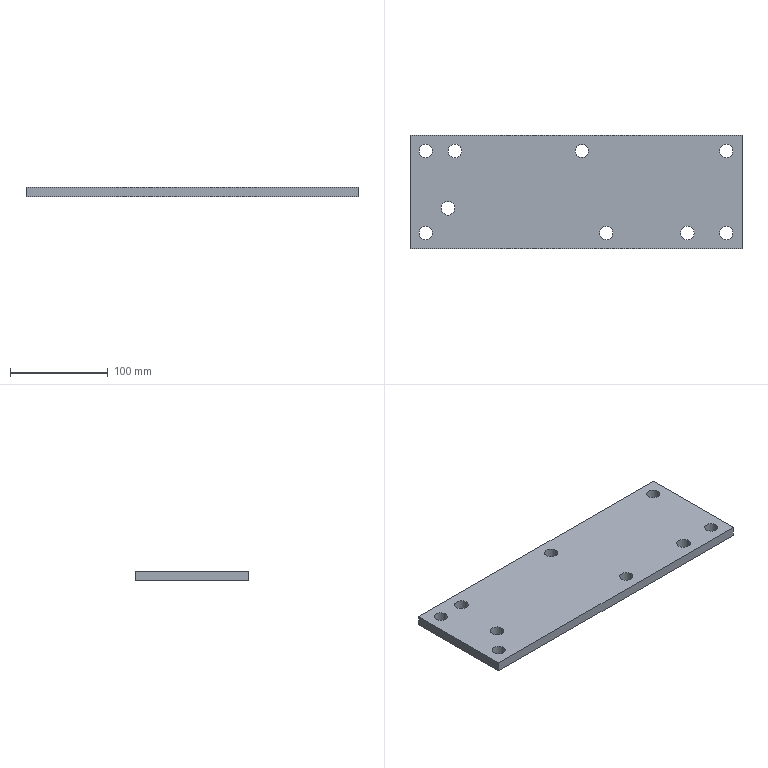Part | NX | features 6 2 | 1 solid | 15 faces | box 340 x 116 x 10 mm | volume 381193 mm3 | cylinder 9 | plane 6 | commonest cylinder face diameters 13.5 x6 14.001 x2 14 x1
STEP:
#1=CARTESIAN_POINT('',(268.029,-411.95,91.));
#2=VERTEX_POINT('',#1);
#3=CARTESIAN_POINT('',(275.029,-411.95,91.));
#4=DIRECTION('',(0.,0.,1.));
#5=DIRECTION('',(-1.,0.,0.));
#6=AXIS2_PLACEMENT_3D('',#3,#4,#5);
#7=CIRCLE('',#6,7.);
#8=EDGE_CURVE('',#2,#2,#7,.T.);
#9=ORIENTED_EDGE('',*,*,#8,.T.);
#10=EDGE_LOOP('',(#9));
#11=FACE_BOUND('',#10,.T.);
#12=CARTESIAN_POINT('',(405.359,-353.223,91.));
#13=VERTEX_POINT('',#12);
#14=CARTESIAN_POINT('',(412.109,-353.223,91.));
#15=DIRECTION('',(0.,0.,-1.));
#16=DIRECTION('',(-1.,0.,0.));
#17=AXIS2_PLACEMENT_3D('',#14,#15,#16);
#18=CIRCLE('',#17,6.75);
#19=EDGE_CURVE('',#13,#13,#18,.T.);
#20=ORIENTED_EDGE('',*,*,#19,.F.);
#21=EDGE_LOOP('',(#20));
#22=FACE_BOUND('',#21,.T.);
#23=CARTESIAN_POINT('',(430.359,-437.223,91.));
#24=VERTEX_POINT('',#23);
#25=CARTESIAN_POINT('',(437.109,-437.223,91.));
#26=DIRECTION('',(0.,0.,-1.));
#27=DIRECTION('',(-1.,0.,0.));
#28=AXIS2_PLACEMENT_3D('',#25,#26,#27);
#29=CIRCLE('',#28,6.75);
#30=EDGE_CURVE('',#24,#24,#29,.T.);
#31=ORIENTED_EDGE('',*,*,#30,.F.);
#32=EDGE_LOOP('',(#31));
#33=FACE_BOUND('',#32,.T.);
#34=CARTESIAN_POINT('',(289.11,-353.223,91.));
#35=VERTEX_POINT('',#34);
#36=CARTESIAN_POINT('',(282.109,-353.223,91.));
#37=DIRECTION('',(0.,0.,-1.));
#38=DIRECTION('',(1.,0.,0.));
#39=AXIS2_PLACEMENT_3D('',#36,#37,#38);
#40=CIRCLE('',#39,7.);
#41=EDGE_CURVE('',#35,#35,#40,.T.);
#42=ORIENTED_EDGE('',*,*,#41,.F.);
#43=EDGE_LOOP('',(#42));
#44=FACE_BOUND('',#43,.T.);
#45=CARTESIAN_POINT('',(566.859,-353.223,91.));
#46=VERTEX_POINT('',#45);
#47=CARTESIAN_POINT('',(560.109,-353.223,91.));
#48=DIRECTION('',(0.,0.,-1.));
#49=DIRECTION('',(1.,0.,0.));
#50=AXIS2_PLACEMENT_3D('',#47,#48,#49);
#51=CIRCLE('',#50,6.75);
#52=EDGE_CURVE('',#46,#46,#51,.T.);
#53=ORIENTED_EDGE('',*,*,#52,.F.);
#54=EDGE_LOOP('',(#53));
#55=FACE_BOUND('',#54,.T.);
#56=CARTESIAN_POINT('',(258.859,-353.223,91.));
#57=VERTEX_POINT('',#56);
#58=CARTESIAN_POINT('',(252.109,-353.223,91.));
#59=DIRECTION('',(0.,0.,-1.));
#60=DIRECTION('',(1.,0.,0.));
#61=AXIS2_PLACEMENT_3D('',#58,#59,#60);
#62=CIRCLE('',#61,6.75);
#63=EDGE_CURVE('',#57,#57,#62,.T.);
#64=ORIENTED_EDGE('',*,*,#63,.F.);
#65=EDGE_LOOP('',(#64));
#66=FACE_BOUND('',#65,.T.);
#67=CARTESIAN_POINT('',(576.109,-337.223,91.));
#68=VERTEX_POINT('',#67);
#69=CARTESIAN_POINT('',(576.109,-453.223,91.));
#70=VERTEX_POINT('',#69);
#71=CARTESIAN_POINT('',(576.109,-392.723,91.));
#72=DIRECTION('',(0.,-1.,0.));
#73=VECTOR('',#72,1000.);
#74=LINE('',#71,#73);
#75=EDGE_CURVE('',#68,#70,#74,.T.);
#76=ORIENTED_EDGE('',*,*,#75,.T.);
#77=CARTESIAN_POINT('',(236.109,-453.223,91.));
#78=VERTEX_POINT('',#77);
#79=CARTESIAN_POINT('',(433.109,-453.223,91.));
#80=DIRECTION('',(-1.,0.,0.));
#81=VECTOR('',#80,1000.);
#82=LINE('',#79,#81);
#83=EDGE_CURVE('',#70,#78,#82,.T.);
#84=ORIENTED_EDGE('',*,*,#83,.T.);
#85=CARTESIAN_POINT('',(236.109,-337.223,91.));
#86=VERTEX_POINT('',#85);
#87=CARTESIAN_POINT('',(236.109,-392.723,91.));
#88=DIRECTION('',(0.,1.,0.));
#89=VECTOR('',#88,1000.);
#90=LINE('',#87,#89);
#91=EDGE_CURVE('',#78,#86,#90,.T.);
#92=ORIENTED_EDGE('',*,*,#91,.T.);
#93=CARTESIAN_POINT('',(433.109,-337.223,91.));
#94=DIRECTION('',(1.,0.,0.));
#95=VECTOR('',#94,1000.);
#96=LINE('',#93,#95);
#97=EDGE_CURVE('',#86,#68,#96,.T.);
#98=ORIENTED_EDGE('',*,*,#97,.T.);
#99=EDGE_LOOP('',(#76,#84,#92,#98));
#100=FACE_BOUND('',#99,.T.);
#101=CARTESIAN_POINT('',(566.859,-437.223,91.));
#102=VERTEX_POINT('',#101);
#103=CARTESIAN_POINT('',(560.109,-437.223,91.));
#104=DIRECTION('',(0.,0.,-1.));
#105=DIRECTION('',(1.,0.,0.));
#106=AXIS2_PLACEMENT_3D('',#103,#104,#105);
#107=CIRCLE('',#106,6.75);
#108=EDGE_CURVE('',#102,#102,#107,.T.);
#109=ORIENTED_EDGE('',*,*,#108,.F.);
#110=EDGE_LOOP('',(#109));
#111=FACE_BOUND('',#110,.T.);
#112=CARTESIAN_POINT('',(258.859,-437.223,91.));
#113=VERTEX_POINT('',#112);
#114=CARTESIAN_POINT('',(252.109,-437.223,91.));
#115=DIRECTION('',(0.,0.,-1.));
#116=DIRECTION('',(1.,0.,0.));
#117=AXIS2_PLACEMENT_3D('',#114,#115,#116);
#118=CIRCLE('',#117,6.75);
#119=EDGE_CURVE('',#113,#113,#118,.T.);
#120=ORIENTED_EDGE('',*,*,#119,.F.);
#121=EDGE_LOOP('',(#120));
#122=FACE_BOUND('',#121,.T.);
#123=CARTESIAN_POINT('',(527.11,-437.223,91.));
#124=VERTEX_POINT('',#123);
#125=CARTESIAN_POINT('',(520.109,-437.223,91.));
#126=DIRECTION('',(0.,0.,-1.));
#127=DIRECTION('',(1.,0.,0.));
#128=AXIS2_PLACEMENT_3D('',#125,#126,#127);
#129=CIRCLE('',#128,7.);
#130=EDGE_CURVE('',#124,#124,#129,.T.);
#131=ORIENTED_EDGE('',*,*,#130,.F.);
#132=EDGE_LOOP('',(#131));
#133=FACE_BOUND('',#132,.T.);
#134=CARTESIAN_POINT('',(433.109,-392.723,91.));
#135=DIRECTION('',(0.,0.,-1.));
#136=DIRECTION('',(1.,0.,0.));
#137=AXIS2_PLACEMENT_3D('',#134,#135,#136);
#138=PLANE('',#137);
#139=ADVANCED_FACE('',(#11,#22,#33,#44,#55,#66,#100,#111,#122,#133),#138,.T.);
#140=CARTESIAN_POINT('',(282.029,-411.95,101.));
#141=VERTEX_POINT('',#140);
#142=CARTESIAN_POINT('',(275.029,-411.95,101.));
#143=DIRECTION('',(0.,0.,-1.));
#144=DIRECTION('',(1.,0.,0.));
#145=AXIS2_PLACEMENT_3D('',#142,#143,#144);
#146=CIRCLE('',#145,7.);
#147=EDGE_CURVE('',#141,#141,#146,.T.);
#148=ORIENTED_EDGE('',*,*,#147,.T.);
#149=EDGE_LOOP('',(#148));
#150=FACE_BOUND('',#149,.T.);
#151=CARTESIAN_POINT('',(418.859,-353.223,101.));
#152=VERTEX_POINT('',#151);
#153=CARTESIAN_POINT('',(412.109,-353.223,101.));
#154=DIRECTION('',(0.,0.,1.));
#155=DIRECTION('',(1.,0.,0.));
#156=AXIS2_PLACEMENT_3D('',#153,#154,#155);
#157=CIRCLE('',#156,6.75);
#158=EDGE_CURVE('',#152,#152,#157,.T.);
#159=ORIENTED_EDGE('',*,*,#158,.F.);
#160=EDGE_LOOP('',(#159));
#161=FACE_BOUND('',#160,.T.);
#162=CARTESIAN_POINT('',(443.859,-437.223,101.));
#163=VERTEX_POINT('',#162);
#164=CARTESIAN_POINT('',(437.109,-437.223,101.));
#165=DIRECTION('',(0.,0.,1.));
#166=DIRECTION('',(1.,0.,0.));
#167=AXIS2_PLACEMENT_3D('',#164,#165,#166);
#168=CIRCLE('',#167,6.75);
#169=EDGE_CURVE('',#163,#163,#168,.T.);
#170=ORIENTED_EDGE('',*,*,#169,.F.);
#171=EDGE_LOOP('',(#170));
#172=FACE_BOUND('',#171,.T.);
#173=CARTESIAN_POINT('',(289.11,-353.223,101.));
#174=VERTEX_POINT('',#173);
#175=CARTESIAN_POINT('',(282.109,-353.223,101.));
#176=DIRECTION('',(0.,0.,1.));
#177=DIRECTION('',(1.,0.,0.));
#178=AXIS2_PLACEMENT_3D('',#175,#176,#177);
#179=CIRCLE('',#178,7.);
#180=EDGE_CURVE('',#174,#174,#179,.T.);
#181=ORIENTED_EDGE('',*,*,#180,.F.);
#182=EDGE_LOOP('',(#181));
#183=FACE_BOUND('',#182,.T.);
#184=CARTESIAN_POINT('',(566.859,-353.223,101.));
#185=VERTEX_POINT('',#184);
#186=CARTESIAN_POINT('',(560.109,-353.223,101.));
#187=DIRECTION('',(0.,0.,1.));
#188=DIRECTION('',(1.,0.,0.));
#189=AXIS2_PLACEMENT_3D('',#186,#187,#188);
#190=CIRCLE('',#189,6.75);
#191=EDGE_CURVE('',#185,#185,#190,.T.);
#192=ORIENTED_EDGE('',*,*,#191,.F.);
#193=EDGE_LOOP('',(#192));
#194=FACE_BOUND('',#193,.T.);
#195=CARTESIAN_POINT('',(258.859,-353.223,101.));
#196=VERTEX_POINT('',#195);
#197=CARTESIAN_POINT('',(252.109,-353.223,101.));
#198=DIRECTION('',(0.,0.,1.));
#199=DIRECTION('',(1.,0.,0.));
#200=AXIS2_PLACEMENT_3D('',#197,#198,#199);
#201=CIRCLE('',#200,6.75);
#202=EDGE_CURVE('',#196,#196,#201,.T.);
#203=ORIENTED_EDGE('',*,*,#202,.F.);
#204=EDGE_LOOP('',(#203));
#205=FACE_BOUND('',#204,.T.);
#206=CARTESIAN_POINT('',(576.109,-337.223,101.));
#207=VERTEX_POINT('',#206);
#208=CARTESIAN_POINT('',(236.109,-337.223,101.));
#209=VERTEX_POINT('',#208);
#210=CARTESIAN_POINT('',(433.109,-337.223,101.));
#211=DIRECTION('',(-1.,0.,0.));
#212=VECTOR('',#211,1000.);
#213=LINE('',#210,#212);
#214=EDGE_CURVE('',#207,#209,#213,.T.);
#215=ORIENTED_EDGE('',*,*,#214,.T.);
#216=CARTESIAN_POINT('',(236.109,-453.223,101.));
#217=VERTEX_POINT('',#216);
#218=CARTESIAN_POINT('',(236.109,-392.723,101.));
#219=DIRECTION('',(0.,-1.,0.));
#220=VECTOR('',#219,1000.);
#221=LINE('',#218,#220);
#222=EDGE_CURVE('',#209,#217,#221,.T.);
#223=ORIENTED_EDGE('',*,*,#222,.T.);
#224=CARTESIAN_POINT('',(576.109,-453.223,101.));
#225=VERTEX_POINT('',#224);
#226=CARTESIAN_POINT('',(433.109,-453.223,101.));
#227=DIRECTION('',(1.,0.,0.));
#228=VECTOR('',#227,1000.);
#229=LINE('',#226,#228);
#230=EDGE_CURVE('',#217,#225,#229,.T.);
#231=ORIENTED_EDGE('',*,*,#230,.T.);
#232=CARTESIAN_POINT('',(576.109,-392.723,101.));
#233=DIRECTION('',(0.,1.,0.));
#234=VECTOR('',#233,1000.);
#235=LINE('',#232,#234);
#236=EDGE_CURVE('',#225,#207,#235,.T.);
#237=ORIENTED_EDGE('',*,*,#236,.T.);
#238=EDGE_LOOP('',(#215,#223,#231,#237));
#239=FACE_BOUND('',#238,.T.);
#240=CARTESIAN_POINT('',(566.859,-437.223,101.));
#241=VERTEX_POINT('',#240);
#242=CARTESIAN_POINT('',(560.109,-437.223,101.));
#243=DIRECTION('',(0.,0.,1.));
#244=DIRECTION('',(1.,0.,0.));
#245=AXIS2_PLACEMENT_3D('',#242,#243,#244);
#246=CIRCLE('',#245,6.75);
#247=EDGE_CURVE('',#241,#241,#246,.T.);
#248=ORIENTED_EDGE('',*,*,#247,.F.);
#249=EDGE_LOOP('',(#248));
#250=FACE_BOUND('',#249,.T.);
#251=CARTESIAN_POINT('',(258.859,-437.223,101.));
#252=VERTEX_POINT('',#251);
#253=CARTESIAN_POINT('',(252.109,-437.223,101.));
#254=DIRECTION('',(0.,0.,1.));
#255=DIRECTION('',(1.,0.,0.));
#256=AXIS2_PLACEMENT_3D('',#253,#254,#255);
#257=CIRCLE('',#256,6.75);
#258=EDGE_CURVE('',#252,#252,#257,.T.);
#259=ORIENTED_EDGE('',*,*,#258,.F.);
#260=EDGE_LOOP('',(#259));
#261=FACE_BOUND('',#260,.T.);
#262=CARTESIAN_POINT('',(527.11,-437.223,101.));
#263=VERTEX_POINT('',#262);
#264=CARTESIAN_POINT('',(520.109,-437.223,101.));
#265=DIRECTION('',(0.,0.,1.));
#266=DIRECTION('',(1.,0.,0.));
#267=AXIS2_PLACEMENT_3D('',#264,#265,#266);
#268=CIRCLE('',#267,7.);
#269=EDGE_CURVE('',#263,#263,#268,.T.);
#270=ORIENTED_EDGE('',*,*,#269,.F.);
#271=EDGE_LOOP('',(#270));
#272=FACE_BOUND('',#271,.T.);
#273=CARTESIAN_POINT('',(-273.37,-123.939,101.));
#274=DIRECTION('',(0.,0.,1.));
#275=DIRECTION('',(-1.,0.,0.));
#276=AXIS2_PLACEMENT_3D('',#273,#274,#275);
#277=PLANE('',#276);
#278=ADVANCED_FACE('',(#150,#161,#172,#183,#194,#205,#239,#250,#261,#272),#277,.T.);
#279=ORIENTED_EDGE('',*,*,#269,.T.);
#280=EDGE_LOOP('',(#279));
#281=FACE_BOUND('',#280,.T.);
#282=ORIENTED_EDGE('',*,*,#130,.T.);
#283=EDGE_LOOP('',(#282));
#284=FACE_BOUND('',#283,.T.);
#285=CARTESIAN_POINT('',(520.109,-437.223,91.));
#286=DIRECTION('',(0.,0.,1.));
#287=DIRECTION('',(-1.,0.,0.));
#288=AXIS2_PLACEMENT_3D('',#285,#286,#287);
#289=CYLINDRICAL_SURFACE('',#288,7.);
#290=ADVANCED_FACE('',(#281,#284),#289,.F.);
#291=ORIENTED_EDGE('',*,*,#258,.T.);
#292=EDGE_LOOP('',(#291));
#293=FACE_BOUND('',#292,.T.);
#294=ORIENTED_EDGE('',*,*,#119,.T.);
#295=EDGE_LOOP('',(#294));
#296=FACE_BOUND('',#295,.T.);
#297=CARTESIAN_POINT('',(252.109,-437.223,91.));
#298=DIRECTION('',(0.,0.,1.));
#299=DIRECTION('',(-1.,0.,0.));
#300=AXIS2_PLACEMENT_3D('',#297,#298,#299);
#301=CYLINDRICAL_SURFACE('',#300,6.75);
#302=ADVANCED_FACE('',(#293,#296),#301,.F.);
#303=ORIENTED_EDGE('',*,*,#247,.T.);
#304=EDGE_LOOP('',(#303));
#305=FACE_BOUND('',#304,.T.);
#306=ORIENTED_EDGE('',*,*,#108,.T.);
#307=EDGE_LOOP('',(#306));
#308=FACE_BOUND('',#307,.T.);
#309=CARTESIAN_POINT('',(560.109,-437.223,91.));
#310=DIRECTION('',(0.,0.,1.));
#311=DIRECTION('',(-1.,0.,0.));
#312=AXIS2_PLACEMENT_3D('',#309,#310,#311);
#313=CYLINDRICAL_SURFACE('',#312,6.75);
#314=ADVANCED_FACE('',(#305,#308),#313,.F.);
#315=CARTESIAN_POINT('',(576.109,-337.223,91.));
#316=DIRECTION('',(0.,0.,1.));
#317=VECTOR('',#316,1000.);
#318=LINE('',#315,#317);
#319=EDGE_CURVE('',#68,#207,#318,.T.);
#320=ORIENTED_EDGE('',*,*,#319,.F.);
#321=ORIENTED_EDGE('',*,*,#97,.F.);
#322=CARTESIAN_POINT('',(236.109,-337.223,91.));
#323=DIRECTION('',(0.,0.,1.));
#324=VECTOR('',#323,1000.);
#325=LINE('',#322,#324);
#326=EDGE_CURVE('',#86,#209,#325,.T.);
#327=ORIENTED_EDGE('',*,*,#326,.T.);
#328=ORIENTED_EDGE('',*,*,#214,.F.);
#329=EDGE_LOOP('',(#320,#321,#327,#328));
#330=FACE_BOUND('',#329,.T.);
#331=CARTESIAN_POINT('',(433.109,-337.223,91.));
#332=DIRECTION('',(0.,1.,0.));
#333=DIRECTION('',(0.,0.,1.));
#334=AXIS2_PLACEMENT_3D('',#331,#332,#333);
#335=PLANE('',#334);
#336=ADVANCED_FACE('',(#330),#335,.T.);
#337=ORIENTED_EDGE('',*,*,#326,.F.);
#338=ORIENTED_EDGE('',*,*,#91,.F.);
#339=CARTESIAN_POINT('',(236.109,-453.223,91.));
#340=DIRECTION('',(0.,0.,1.));
#341=VECTOR('',#340,1000.);
#342=LINE('',#339,#341);
#343=EDGE_CURVE('',#78,#217,#342,.T.);
#344=ORIENTED_EDGE('',*,*,#343,.T.);
#345=ORIENTED_EDGE('',*,*,#222,.F.);
#346=EDGE_LOOP('',(#337,#338,#344,#345));
#347=FACE_BOUND('',#346,.T.);
#348=CARTESIAN_POINT('',(236.109,-392.723,91.));
#349=DIRECTION('',(-1.,0.,0.));
#350=DIRECTION('',(0.,0.,-1.));
#351=AXIS2_PLACEMENT_3D('',#348,#349,#350);
#352=PLANE('',#351);
#353=ADVANCED_FACE('',(#347),#352,.T.);
#354=ORIENTED_EDGE('',*,*,#343,.F.);
#355=ORIENTED_EDGE('',*,*,#83,.F.);
#356=CARTESIAN_POINT('',(576.109,-453.223,91.));
#357=DIRECTION('',(0.,0.,1.));
#358=VECTOR('',#357,1000.);
#359=LINE('',#356,#358);
#360=EDGE_CURVE('',#70,#225,#359,.T.);
#361=ORIENTED_EDGE('',*,*,#360,.T.);
#362=ORIENTED_EDGE('',*,*,#230,.F.);
#363=EDGE_LOOP('',(#354,#355,#361,#362));
#364=FACE_BOUND('',#363,.T.);
#365=CARTESIAN_POINT('',(433.109,-453.223,91.));
#366=DIRECTION('',(0.,-1.,0.));
#367=DIRECTION('',(0.,0.,-1.));
#368=AXIS2_PLACEMENT_3D('',#365,#366,#367);
#369=PLANE('',#368);
#370=ADVANCED_FACE('',(#364),#369,.T.);
#371=ORIENTED_EDGE('',*,*,#75,.F.);
#372=ORIENTED_EDGE('',*,*,#319,.T.);
#373=ORIENTED_EDGE('',*,*,#236,.F.);
#374=ORIENTED_EDGE('',*,*,#360,.F.);
#375=EDGE_LOOP('',(#371,#372,#373,#374));
#376=FACE_BOUND('',#375,.T.);
#377=CARTESIAN_POINT('',(576.109,-392.723,91.));
#378=DIRECTION('',(1.,0.,0.));
#379=DIRECTION('',(0.,0.,1.));
#380=AXIS2_PLACEMENT_3D('',#377,#378,#379);
#381=PLANE('',#380);
#382=ADVANCED_FACE('',(#376),#381,.T.);
#383=ORIENTED_EDGE('',*,*,#202,.T.);
#384=EDGE_LOOP('',(#383));
#385=FACE_BOUND('',#384,.T.);
#386=ORIENTED_EDGE('',*,*,#63,.T.);
#387=EDGE_LOOP('',(#386));
#388=FACE_BOUND('',#387,.T.);
#389=CARTESIAN_POINT('',(252.109,-353.223,91.));
#390=DIRECTION('',(0.,0.,1.));
#391=DIRECTION('',(-1.,0.,0.));
#392=AXIS2_PLACEMENT_3D('',#389,#390,#391);
#393=CYLINDRICAL_SURFACE('',#392,6.75);
#394=ADVANCED_FACE('',(#385,#388),#393,.F.);
#395=ORIENTED_EDGE('',*,*,#191,.T.);
#396=EDGE_LOOP('',(#395));
#397=FACE_BOUND('',#396,.T.);
#398=ORIENTED_EDGE('',*,*,#52,.T.);
#399=EDGE_LOOP('',(#398));
#400=FACE_BOUND('',#399,.T.);
#401=CARTESIAN_POINT('',(560.109,-353.223,91.));
#402=DIRECTION('',(0.,0.,1.));
#403=DIRECTION('',(-1.,0.,0.));
#404=AXIS2_PLACEMENT_3D('',#401,#402,#403);
#405=CYLINDRICAL_SURFACE('',#404,6.75);
#406=ADVANCED_FACE('',(#397,#400),#405,.F.);
#407=ORIENTED_EDGE('',*,*,#180,.T.);
#408=EDGE_LOOP('',(#407));
#409=FACE_BOUND('',#408,.T.);
#410=ORIENTED_EDGE('',*,*,#41,.T.);
#411=EDGE_LOOP('',(#410));
#412=FACE_BOUND('',#411,.T.);
#413=CARTESIAN_POINT('',(282.109,-353.223,91.));
#414=DIRECTION('',(0.,0.,1.));
#415=DIRECTION('',(-1.,0.,0.));
#416=AXIS2_PLACEMENT_3D('',#413,#414,#415);
#417=CYLINDRICAL_SURFACE('',#416,7.);
#418=ADVANCED_FACE('',(#409,#412),#417,.F.);
#419=ORIENTED_EDGE('',*,*,#169,.T.);
#420=EDGE_LOOP('',(#419));
#421=FACE_BOUND('',#420,.T.);
#422=ORIENTED_EDGE('',*,*,#30,.T.);
#423=EDGE_LOOP('',(#422));
#424=FACE_BOUND('',#423,.T.);
#425=CARTESIAN_POINT('',(437.109,-437.223,91.));
#426=DIRECTION('',(0.,0.,1.));
#427=DIRECTION('',(-1.,0.,0.));
#428=AXIS2_PLACEMENT_3D('',#425,#426,#427);
#429=CYLINDRICAL_SURFACE('',#428,6.75);
#430=ADVANCED_FACE('',(#421,#424),#429,.F.);
#431=ORIENTED_EDGE('',*,*,#158,.T.);
#432=EDGE_LOOP('',(#431));
#433=FACE_BOUND('',#432,.T.);
#434=ORIENTED_EDGE('',*,*,#19,.T.);
#435=EDGE_LOOP('',(#434));
#436=FACE_BOUND('',#435,.T.);
#437=CARTESIAN_POINT('',(412.109,-353.223,91.));
#438=DIRECTION('',(0.,0.,1.));
#439=DIRECTION('',(-1.,0.,0.));
#440=AXIS2_PLACEMENT_3D('',#437,#438,#439);
#441=CYLINDRICAL_SURFACE('',#440,6.75);
#442=ADVANCED_FACE('',(#433,#436),#441,.F.);
#443=ORIENTED_EDGE('',*,*,#8,.F.);
#444=EDGE_LOOP('',(#443));
#445=FACE_BOUND('',#444,.T.);
#446=ORIENTED_EDGE('',*,*,#147,.F.);
#447=EDGE_LOOP('',(#446));
#448=FACE_BOUND('',#447,.T.);
#449=CARTESIAN_POINT('',(275.029,-411.95,-138.15));
#450=DIRECTION('',(0.,0.,1.));
#451=DIRECTION('',(-1.,0.,0.));
#452=AXIS2_PLACEMENT_3D('',#449,#450,#451);
#453=CYLINDRICAL_SURFACE('',#452,7.);
#454=ADVANCED_FACE('',(#445,#448),#453,.F.);
#455=CLOSED_SHELL('',(#139,#278,#290,#302,#314,#336,#353,#370,#382,#394,#406,#418,#430,#442,#454));
#456=MANIFOLD_SOLID_BREP('',#455);
#457=(LENGTH_UNIT()NAMED_UNIT(*)SI_UNIT(.MILLI.,.METRE.));
#458=UNCERTAINTY_MEASURE_WITH_UNIT(LENGTH_MEASURE(0.00001),#457,'','');
#459=(NAMED_UNIT(*)PLANE_ANGLE_UNIT()SI_UNIT($,.RADIAN.));
#460=(NAMED_UNIT(*)SI_UNIT($,.STERADIAN.)SOLID_ANGLE_UNIT());
#461=(GEOMETRIC_REPRESENTATION_CONTEXT(3)GLOBAL_UNCERTAINTY_ASSIGNED_CONTEXT((#458))GLOBAL_UNIT_ASSIGNED_CONTEXT((#457,#459,#460))REPRESENTATION_CONTEXT('',''));
#462=ADVANCED_BREP_SHAPE_REPRESENTATION('',(#456),#461);